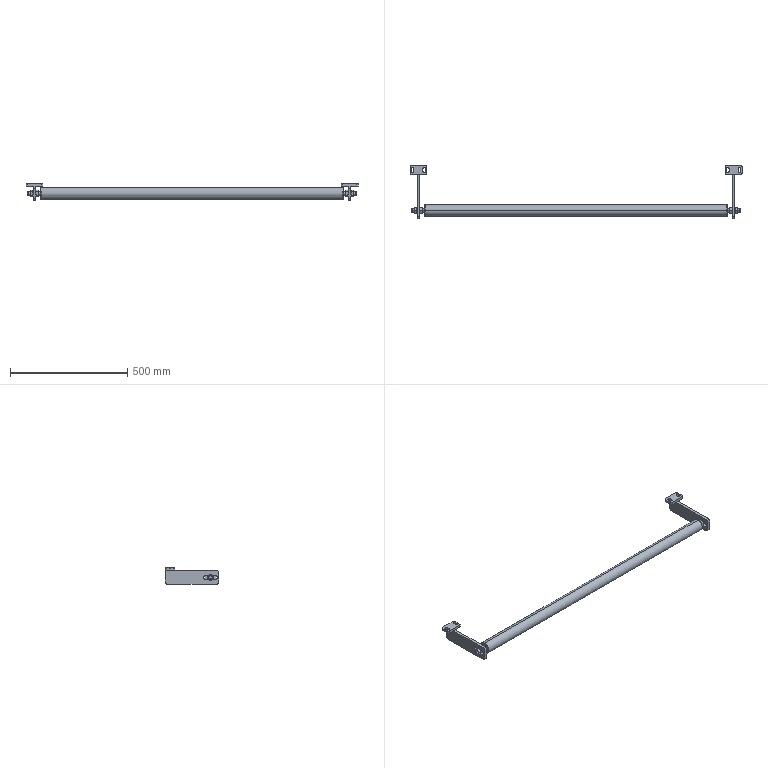Part | SolidWorks | features BaseBody 9 | 9 solids | 224 faces | box 1417 x 228 x 72 mm | volume 2932571 mm3 | plane 120 | cone 64 | cylinder 40 | commonest cylinder face diameters 16 x12 10 x8 12 x8 20 x6 17 x4 50 x2